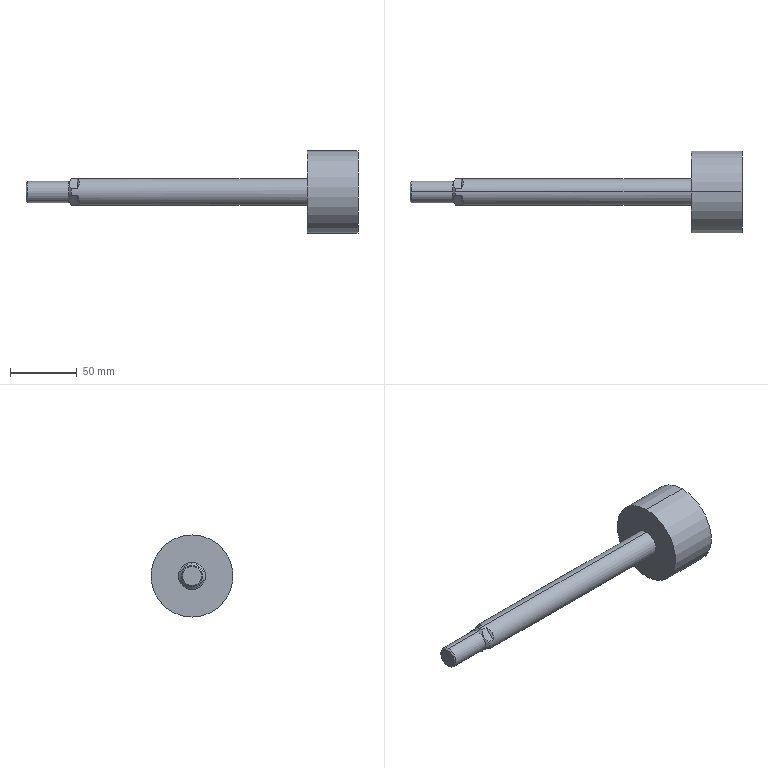Part | SolidWorks | features BaseBody 1 | 1 solid | 21 faces | box 248.5 x 61.5 x 61.5 mm | volume 175012 mm3 | plane 11 | cylinder 6 | cone 4 | commonest cylinder face diameters 16 x2 20 x2 61.5 x2
STEP:
#1=CARTESIAN_POINT('',(-37.,0.,-8.));
#2=VERTEX_POINT('',#1);
#3=CARTESIAN_POINT('',(-37.,0.,8.));
#4=VERTEX_POINT('',#3);
#5=CARTESIAN_POINT('',(-37.,0.,0.));
#6=DIRECTION('',(1.,0.,0.));
#7=DIRECTION('',(0.,0.,-1.));
#8=AXIS2_PLACEMENT_3D('',#5,#6,#7);
#9=CIRCLE('',#8,8.);
#10=EDGE_CURVE('',#2,#4,#9,.T.);
#11=ORIENTED_EDGE('',*,*,#10,.T.);
#12=CARTESIAN_POINT('',(-35.,0.,10.));
#13=VERTEX_POINT('',#12);
#14=CARTESIAN_POINT('',(-37.,0.,8.));
#15=DIRECTION('',(0.7071,0.,0.7071));
#16=VECTOR('',#15,1000.);
#17=LINE('',#14,#16);
#18=EDGE_CURVE('',#4,#13,#17,.T.);
#19=ORIENTED_EDGE('',*,*,#18,.T.);
#20=CARTESIAN_POINT('',(-35.,2.285,9.735));
#21=VERTEX_POINT('',#20);
#22=CARTESIAN_POINT('',(-35.,0.,0.));
#23=DIRECTION('',(1.,0.,0.));
#24=DIRECTION('',(0.,0.,-1.));
#25=AXIS2_PLACEMENT_3D('',#22,#23,#24);
#26=CIRCLE('',#25,10.);
#27=EDGE_CURVE('',#21,#13,#26,.T.);
#28=ORIENTED_EDGE('',*,*,#27,.F.);
#29=CARTESIAN_POINT('',(-35.,9.735,2.285));
#30=VERTEX_POINT('',#29);
#31=CARTESIAN_POINT('',(-35.,9.735,2.285));
#32=CARTESIAN_POINT('',(-35.236,9.419,2.602));
#33=CARTESIAN_POINT('',(-35.546,8.958,3.063));
#34=CARTESIAN_POINT('',(-35.834,8.441,3.58));
#35=CARTESIAN_POINT('',(-35.96,8.189,3.832));
#36=CARTESIAN_POINT('',(-36.018,8.064,3.957));
#37=CARTESIAN_POINT('',(-36.046,8.001,4.019));
#38=CARTESIAN_POINT('',(-36.057,7.975,4.046));
#39=CARTESIAN_POINT('',(-36.065,7.957,4.064));
#40=CARTESIAN_POINT('',(-36.068,7.95,4.071));
#41=CARTESIAN_POINT('',(-36.357,7.281,4.74));
#42=CARTESIAN_POINT('',(-36.5,6.638,5.383));
#43=CARTESIAN_POINT('',(-36.5,5.698,6.323));
#44=CARTESIAN_POINT('',(-36.447,5.221,6.799));
#45=CARTESIAN_POINT('',(-36.291,4.655,7.365));
#46=CARTESIAN_POINT('',(-36.19,4.37,7.651));
#47=CARTESIAN_POINT('',(-36.134,4.226,7.795));
#48=CARTESIAN_POINT('',(-36.104,4.154,7.866));
#49=CARTESIAN_POINT('',(-36.091,4.124,7.897));
#50=CARTESIAN_POINT('',(-36.082,4.103,7.918));
#51=CARTESIAN_POINT('',(-36.077,4.091,7.93));
#52=CARTESIAN_POINT('',(-35.829,3.517,8.503));
#53=CARTESIAN_POINT('',(-35.472,2.919,9.102));
#54=CARTESIAN_POINT('',(-35.,2.285,9.735));
#55=B_SPLINE_CURVE_WITH_KNOTS('',3,(#31,#32,#33,#34,#35,#36,#37,#38,#39,#40,#41,#42,#43,#44,#45,#46,#47,#48,#49,#50,#51,#52,#53,#54),.UNSPECIFIED.,.F.,.F.,(4,1,1,1,1,1,2,2,2,1,1,1,1,1,2,2,4),(0.,0.125,0.1875,0.2188,0.2344,0.2422,0.2461,0.25,0.5,0.625,0.6875,0.7188,0.7344,0.7422,0.7461,0.75,1.),.UNSPECIFIED.);
#56=EDGE_CURVE('',#30,#21,#55,.T.);
#57=ORIENTED_EDGE('',*,*,#56,.F.);
#58=CARTESIAN_POINT('',(-35.,9.735,-2.285));
#59=VERTEX_POINT('',#58);
#60=CARTESIAN_POINT('',(-35.,0.,0.));
#61=DIRECTION('',(1.,0.,0.));
#62=DIRECTION('',(0.,0.,-1.));
#63=AXIS2_PLACEMENT_3D('',#60,#61,#62);
#64=CIRCLE('',#63,10.);
#65=EDGE_CURVE('',#59,#30,#64,.T.);
#66=ORIENTED_EDGE('',*,*,#65,.F.);
#67=CARTESIAN_POINT('',(-35.,2.285,-9.735));
#68=VERTEX_POINT('',#67);
#69=CARTESIAN_POINT('',(-35.,2.285,-9.735));
#70=CARTESIAN_POINT('',(-35.236,2.602,-9.419));
#71=CARTESIAN_POINT('',(-35.546,3.063,-8.958));
#72=CARTESIAN_POINT('',(-35.834,3.58,-8.441));
#73=CARTESIAN_POINT('',(-35.96,3.832,-8.189));
#74=CARTESIAN_POINT('',(-36.018,3.957,-8.064));
#75=CARTESIAN_POINT('',(-36.046,4.019,-8.001));
#76=CARTESIAN_POINT('',(-36.057,4.046,-7.975));
#77=CARTESIAN_POINT('',(-36.065,4.064,-7.957));
#78=CARTESIAN_POINT('',(-36.068,4.071,-7.95));
#79=CARTESIAN_POINT('',(-36.357,4.74,-7.281));
#80=CARTESIAN_POINT('',(-36.5,5.383,-6.638));
#81=CARTESIAN_POINT('',(-36.5,6.323,-5.698));
#82=CARTESIAN_POINT('',(-36.447,6.799,-5.221));
#83=CARTESIAN_POINT('',(-36.291,7.365,-4.655));
#84=CARTESIAN_POINT('',(-36.19,7.651,-4.37));
#85=CARTESIAN_POINT('',(-36.134,7.795,-4.226));
#86=CARTESIAN_POINT('',(-36.104,7.866,-4.154));
#87=CARTESIAN_POINT('',(-36.091,7.897,-4.124));
#88=CARTESIAN_POINT('',(-36.082,7.918,-4.103));
#89=CARTESIAN_POINT('',(-36.077,7.93,-4.091));
#90=CARTESIAN_POINT('',(-35.829,8.503,-3.517));
#91=CARTESIAN_POINT('',(-35.472,9.102,-2.919));
#92=CARTESIAN_POINT('',(-35.,9.735,-2.285));
#93=B_SPLINE_CURVE_WITH_KNOTS('',3,(#69,#70,#71,#72,#73,#74,#75,#76,#77,#78,#79,#80,#81,#82,#83,#84,#85,#86,#87,#88,#89,#90,#91,#92),.UNSPECIFIED.,.F.,.F.,(4,1,1,1,1,1,2,2,2,1,1,1,1,1,2,2,4),(0.,0.125,0.1875,0.2188,0.2344,0.2422,0.2461,0.25,0.5,0.625,0.6875,0.7188,0.7344,0.7422,0.7461,0.75,1.),.UNSPECIFIED.);
#94=EDGE_CURVE('',#68,#59,#93,.T.);
#95=ORIENTED_EDGE('',*,*,#94,.F.);
#96=CARTESIAN_POINT('',(-35.,0.,-10.));
#97=VERTEX_POINT('',#96);
#98=CARTESIAN_POINT('',(-35.,0.,0.));
#99=DIRECTION('',(1.,0.,0.));
#100=DIRECTION('',(0.,0.,-1.));
#101=AXIS2_PLACEMENT_3D('',#98,#99,#100);
#102=CIRCLE('',#101,10.);
#103=EDGE_CURVE('',#97,#68,#102,.T.);
#104=ORIENTED_EDGE('',*,*,#103,.F.);
#105=CARTESIAN_POINT('',(-37.,0.,-8.));
#106=DIRECTION('',(0.7071,0.,-0.7071));
#107=VECTOR('',#106,1000.);
#108=LINE('',#105,#107);
#109=EDGE_CURVE('',#2,#97,#108,.T.);
#110=ORIENTED_EDGE('',*,*,#109,.F.);
#111=EDGE_LOOP('',(#11,#19,#28,#57,#66,#95,#104,#110));
#112=FACE_OUTER_BOUND('',#111,.T.);
#113=CARTESIAN_POINT('',(-37.,0.,0.));
#114=DIRECTION('',(1.,0.,0.));
#115=DIRECTION('',(0.,0.,-1.));
#116=AXIS2_PLACEMENT_3D('',#113,#114,#115);
#117=CONICAL_SURFACE('',#116,8.,0.7854);
#118=ADVANCED_FACE('',(#112),#117,.T.);
#119=CARTESIAN_POINT('',(141.5,0.,10.));
#120=VERTEX_POINT('',#119);
#121=CARTESIAN_POINT('',(141.5,0.,-10.));
#122=VERTEX_POINT('',#121);
#123=CARTESIAN_POINT('',(141.5,0.,0.));
#124=DIRECTION('',(1.,0.,0.));
#125=DIRECTION('',(0.,0.,-1.));
#126=AXIS2_PLACEMENT_3D('',#123,#124,#125);
#127=CIRCLE('',#126,10.);
#128=EDGE_CURVE('',#120,#122,#127,.T.);
#129=ORIENTED_EDGE('',*,*,#128,.F.);
#130=CARTESIAN_POINT('',(179.5,0.,10.));
#131=DIRECTION('',(-1.,0.,0.));
#132=VECTOR('',#131,1000.);
#133=LINE('',#130,#132);
#134=EDGE_CURVE('',#120,#13,#133,.T.);
#135=ORIENTED_EDGE('',*,*,#134,.T.);
#136=CARTESIAN_POINT('',(-35.,-2.285,9.735));
#137=VERTEX_POINT('',#136);
#138=CARTESIAN_POINT('',(-35.,0.,0.));
#139=DIRECTION('',(1.,0.,0.));
#140=DIRECTION('',(0.,0.,-1.));
#141=AXIS2_PLACEMENT_3D('',#138,#139,#140);
#142=CIRCLE('',#141,10.);
#143=EDGE_CURVE('',#13,#137,#142,.T.);
#144=ORIENTED_EDGE('',*,*,#143,.T.);
#145=CARTESIAN_POINT('',(-30.5,-2.285,9.735));
#146=VERTEX_POINT('',#145);
#147=CARTESIAN_POINT('',(179.5,-2.285,9.735));
#148=DIRECTION('',(-1.,0.,0.));
#149=VECTOR('',#148,1000.);
#150=LINE('',#147,#149);
#151=EDGE_CURVE('',#146,#137,#150,.T.);
#152=ORIENTED_EDGE('',*,*,#151,.F.);
#153=CARTESIAN_POINT('',(-30.5,-9.735,2.285));
#154=VERTEX_POINT('',#153);
#155=CARTESIAN_POINT('',(-30.5,-9.735,2.285));
#156=CARTESIAN_POINT('',(-28.444,-8.844,6.084));
#157=CARTESIAN_POINT('',(-28.444,-6.084,8.844));
#158=CARTESIAN_POINT('',(-30.5,-2.285,9.735));
#159=(BOUNDED_CURVE()B_SPLINE_CURVE(3,(#155,#156,#157,#158),.UNSPECIFIED.,.F.,.F.)B_SPLINE_CURVE_WITH_KNOTS((4,4),(5.728,6.838),.UNSPECIFIED.)CURVE()GEOMETRIC_REPRESENTATION_ITEM()RATIONAL_B_SPLINE_CURVE((1.,0.9,0.9,1.))REPRESENTATION_ITEM(''));
#160=EDGE_CURVE('',#154,#146,#159,.T.);
#161=ORIENTED_EDGE('',*,*,#160,.F.);
#162=CARTESIAN_POINT('',(-35.,-9.735,2.285));
#163=VERTEX_POINT('',#162);
#164=CARTESIAN_POINT('',(179.5,-9.735,2.285));
#165=DIRECTION('',(1.,0.,0.));
#166=VECTOR('',#165,1000.);
#167=LINE('',#164,#166);
#168=EDGE_CURVE('',#163,#154,#167,.T.);
#169=ORIENTED_EDGE('',*,*,#168,.F.);
#170=CARTESIAN_POINT('',(-35.,-9.735,-2.285));
#171=VERTEX_POINT('',#170);
#172=CARTESIAN_POINT('',(-35.,0.,0.));
#173=DIRECTION('',(1.,0.,0.));
#174=DIRECTION('',(0.,0.,-1.));
#175=AXIS2_PLACEMENT_3D('',#172,#173,#174);
#176=CIRCLE('',#175,10.);
#177=EDGE_CURVE('',#163,#171,#176,.T.);
#178=ORIENTED_EDGE('',*,*,#177,.T.);
#179=CARTESIAN_POINT('',(-30.5,-9.735,-2.285));
#180=VERTEX_POINT('',#179);
#181=CARTESIAN_POINT('',(179.5,-9.735,-2.285));
#182=DIRECTION('',(-1.,0.,0.));
#183=VECTOR('',#182,1000.);
#184=LINE('',#181,#183);
#185=EDGE_CURVE('',#180,#171,#184,.T.);
#186=ORIENTED_EDGE('',*,*,#185,.F.);
#187=CARTESIAN_POINT('',(-30.5,-2.285,-9.735));
#188=VERTEX_POINT('',#187);
#189=CARTESIAN_POINT('',(-30.5,-2.285,-9.735));
#190=CARTESIAN_POINT('',(-28.444,-6.084,-8.844));
#191=CARTESIAN_POINT('',(-28.444,-8.844,-6.084));
#192=CARTESIAN_POINT('',(-30.5,-9.735,-2.285));
#193=(BOUNDED_CURVE()B_SPLINE_CURVE(3,(#189,#190,#191,#192),.UNSPECIFIED.,.F.,.F.)B_SPLINE_CURVE_WITH_KNOTS((4,4),(5.728,6.838),.UNSPECIFIED.)CURVE()GEOMETRIC_REPRESENTATION_ITEM()RATIONAL_B_SPLINE_CURVE((1.,0.9,0.9,1.))REPRESENTATION_ITEM(''));
#194=EDGE_CURVE('',#188,#180,#193,.T.);
#195=ORIENTED_EDGE('',*,*,#194,.F.);
#196=CARTESIAN_POINT('',(-35.,-2.285,-9.735));
#197=VERTEX_POINT('',#196);
#198=CARTESIAN_POINT('',(179.5,-2.285,-9.735));
#199=DIRECTION('',(1.,0.,0.));
#200=VECTOR('',#199,1000.);
#201=LINE('',#198,#200);
#202=EDGE_CURVE('',#197,#188,#201,.T.);
#203=ORIENTED_EDGE('',*,*,#202,.F.);
#204=CARTESIAN_POINT('',(-35.,0.,0.));
#205=DIRECTION('',(1.,0.,0.));
#206=DIRECTION('',(0.,0.,-1.));
#207=AXIS2_PLACEMENT_3D('',#204,#205,#206);
#208=CIRCLE('',#207,10.);
#209=EDGE_CURVE('',#197,#97,#208,.T.);
#210=ORIENTED_EDGE('',*,*,#209,.T.);
#211=CARTESIAN_POINT('',(179.5,0.,-10.));
#212=DIRECTION('',(-1.,0.,0.));
#213=VECTOR('',#212,1000.);
#214=LINE('',#211,#213);
#215=EDGE_CURVE('',#122,#97,#214,.T.);
#216=ORIENTED_EDGE('',*,*,#215,.F.);
#217=EDGE_LOOP('',(#129,#135,#144,#152,#161,#169,#178,#186,#195,#203,#210,#216));
#218=FACE_OUTER_BOUND('',#217,.T.);
#219=CARTESIAN_POINT('',(179.5,0.,0.));
#220=DIRECTION('',(-1.,0.,0.));
#221=DIRECTION('',(0.,0.,-1.));
#222=AXIS2_PLACEMENT_3D('',#219,#220,#221);
#223=CYLINDRICAL_SURFACE('',#222,10.);
#224=ADVANCED_FACE('',(#218),#223,.T.);
#225=CARTESIAN_POINT('',(179.5,0.,30.75));
#226=VERTEX_POINT('',#225);
#227=CARTESIAN_POINT('',(179.5,0.,-30.75));
#228=VERTEX_POINT('',#227);
#229=CARTESIAN_POINT('',(179.5,0.,0.));
#230=DIRECTION('',(1.,0.,0.));
#231=DIRECTION('',(0.,0.,-1.));
#232=AXIS2_PLACEMENT_3D('',#229,#230,#231);
#233=CIRCLE('',#232,30.75);
#234=EDGE_CURVE('',#226,#228,#233,.T.);
#235=ORIENTED_EDGE('',*,*,#234,.F.);
#236=CARTESIAN_POINT('',(141.5,0.,30.75));
#237=VERTEX_POINT('',#236);
#238=CARTESIAN_POINT('',(179.5,0.,30.75));
#239=DIRECTION('',(-1.,0.,0.));
#240=VECTOR('',#239,1000.);
#241=LINE('',#238,#240);
#242=EDGE_CURVE('',#226,#237,#241,.T.);
#243=ORIENTED_EDGE('',*,*,#242,.T.);
#244=CARTESIAN_POINT('',(141.5,0.,-30.75));
#245=VERTEX_POINT('',#244);
#246=CARTESIAN_POINT('',(141.5,0.,0.));
#247=DIRECTION('',(1.,0.,0.));
#248=DIRECTION('',(0.,0.,-1.));
#249=AXIS2_PLACEMENT_3D('',#246,#247,#248);
#250=CIRCLE('',#249,30.75);
#251=EDGE_CURVE('',#237,#245,#250,.T.);
#252=ORIENTED_EDGE('',*,*,#251,.T.);
#253=CARTESIAN_POINT('',(179.5,0.,-30.75));
#254=DIRECTION('',(-1.,0.,0.));
#255=VECTOR('',#254,1000.);
#256=LINE('',#253,#255);
#257=EDGE_CURVE('',#228,#245,#256,.T.);
#258=ORIENTED_EDGE('',*,*,#257,.F.);
#259=EDGE_LOOP('',(#235,#243,#252,#258));
#260=FACE_OUTER_BOUND('',#259,.T.);
#261=CARTESIAN_POINT('',(179.5,0.,0.));
#262=DIRECTION('',(-1.,0.,0.));
#263=DIRECTION('',(0.,0.,-1.));
#264=AXIS2_PLACEMENT_3D('',#261,#262,#263);
#265=CYLINDRICAL_SURFACE('',#264,30.75);
#266=ADVANCED_FACE('',(#260),#265,.T.);
#267=CARTESIAN_POINT('',(-37.,0.,0.));
#268=DIRECTION('',(1.,0.,0.));
#269=DIRECTION('',(0.,0.,-1.));
#270=AXIS2_PLACEMENT_3D('',#267,#268,#269);
#271=CIRCLE('',#270,8.);
#272=EDGE_CURVE('',#4,#2,#271,.T.);
#273=ORIENTED_EDGE('',*,*,#272,.F.);
#274=CARTESIAN_POINT('',(-68.08,0.,8.));
#275=VERTEX_POINT('',#274);
#276=CARTESIAN_POINT('',(179.5,0.,8.));
#277=DIRECTION('',(-1.,0.,0.));
#278=VECTOR('',#277,1000.);
#279=LINE('',#276,#278);
#280=EDGE_CURVE('',#4,#275,#279,.T.);
#281=ORIENTED_EDGE('',*,*,#280,.T.);
#282=CARTESIAN_POINT('',(-68.08,0.,-8.));
#283=VERTEX_POINT('',#282);
#284=CARTESIAN_POINT('',(-68.08,0.,0.));
#285=DIRECTION('',(1.,0.,0.));
#286=DIRECTION('',(0.,0.,-1.));
#287=AXIS2_PLACEMENT_3D('',#284,#285,#286);
#288=CIRCLE('',#287,8.);
#289=EDGE_CURVE('',#275,#283,#288,.T.);
#290=ORIENTED_EDGE('',*,*,#289,.T.);
#291=CARTESIAN_POINT('',(179.5,0.,-8.));
#292=DIRECTION('',(-1.,0.,0.));
#293=VECTOR('',#292,1000.);
#294=LINE('',#291,#293);
#295=EDGE_CURVE('',#2,#283,#294,.T.);
#296=ORIENTED_EDGE('',*,*,#295,.F.);
#297=EDGE_LOOP('',(#273,#281,#290,#296));
#298=FACE_OUTER_BOUND('',#297,.T.);
#299=CARTESIAN_POINT('',(179.5,0.,0.));
#300=DIRECTION('',(-1.,0.,0.));
#301=DIRECTION('',(0.,0.,-1.));
#302=AXIS2_PLACEMENT_3D('',#299,#300,#301);
#303=CYLINDRICAL_SURFACE('',#302,8.);
#304=ADVANCED_FACE('',(#298),#303,.T.);
#305=CARTESIAN_POINT('',(-69.,0.,-7.08));
#306=VERTEX_POINT('',#305);
#307=CARTESIAN_POINT('',(-69.,0.,7.08));
#308=VERTEX_POINT('',#307);
#309=CARTESIAN_POINT('',(-69.,0.,0.));
#310=DIRECTION('',(1.,0.,0.));
#311=DIRECTION('',(0.,0.,-1.));
#312=AXIS2_PLACEMENT_3D('',#309,#310,#311);
#313=CIRCLE('',#312,7.08);
#314=EDGE_CURVE('',#306,#308,#313,.T.);
#315=ORIENTED_EDGE('',*,*,#314,.T.);
#316=CARTESIAN_POINT('',(-69.,0.,7.08));
#317=DIRECTION('',(0.7071,0.,0.7071));
#318=VECTOR('',#317,1000.);
#319=LINE('',#316,#318);
#320=EDGE_CURVE('',#308,#275,#319,.T.);
#321=ORIENTED_EDGE('',*,*,#320,.T.);
#322=CARTESIAN_POINT('',(-68.08,0.,0.));
#323=DIRECTION('',(1.,0.,0.));
#324=DIRECTION('',(0.,0.,-1.));
#325=AXIS2_PLACEMENT_3D('',#322,#323,#324);
#326=CIRCLE('',#325,8.);
#327=EDGE_CURVE('',#283,#275,#326,.T.);
#328=ORIENTED_EDGE('',*,*,#327,.F.);
#329=CARTESIAN_POINT('',(-69.,0.,-7.08));
#330=DIRECTION('',(0.7071,0.,-0.7071));
#331=VECTOR('',#330,1000.);
#332=LINE('',#329,#331);
#333=EDGE_CURVE('',#306,#283,#332,.T.);
#334=ORIENTED_EDGE('',*,*,#333,.F.);
#335=EDGE_LOOP('',(#315,#321,#328,#334));
#336=FACE_OUTER_BOUND('',#335,.T.);
#337=CARTESIAN_POINT('',(-69.,0.,0.));
#338=DIRECTION('',(1.,0.,0.));
#339=DIRECTION('',(0.,0.,-1.));
#340=AXIS2_PLACEMENT_3D('',#337,#338,#339);
#341=CONICAL_SURFACE('',#340,7.08,0.7854);
#342=ADVANCED_FACE('',(#336),#341,.T.);
#343=CARTESIAN_POINT('',(-30.5,2.285,9.735));
#344=VERTEX_POINT('',#343);
#345=CARTESIAN_POINT('',(179.5,2.285,9.735));
#346=DIRECTION('',(1.,0.,0.));
#347=VECTOR('',#346,1000.);
#348=LINE('',#345,#347);
#349=EDGE_CURVE('',#21,#344,#348,.T.);
#350=ORIENTED_EDGE('',*,*,#349,.T.);
#351=CARTESIAN_POINT('',(-30.5,9.735,2.285));
#352=VERTEX_POINT('',#351);
#353=CARTESIAN_POINT('',(-30.5,0.,12.021));
#354=DIRECTION('',(0.,0.7071,-0.7071));
#355=VECTOR('',#354,1000.);
#356=LINE('',#353,#355);
#357=EDGE_CURVE('',#344,#352,#356,.T.);
#358=ORIENTED_EDGE('',*,*,#357,.T.);
#359=CARTESIAN_POINT('',(179.5,9.735,2.285));
#360=DIRECTION('',(-1.,0.,0.));
#361=VECTOR('',#360,1000.);
#362=LINE('',#359,#361);
#363=EDGE_CURVE('',#352,#30,#362,.T.);
#364=ORIENTED_EDGE('',*,*,#363,.T.);
#365=ORIENTED_EDGE('',*,*,#56,.T.);
#366=EDGE_LOOP('',(#350,#358,#364,#365));
#367=FACE_OUTER_BOUND('',#366,.T.);
#368=CARTESIAN_POINT('',(-71.7,0.,12.021));
#369=DIRECTION('',(0.,0.7071,0.7071));
#370=DIRECTION('',(1.,0.,0.));
#371=AXIS2_PLACEMENT_3D('',#368,#369,#370);
#372=PLANE('',#371);
#373=ADVANCED_FACE('',(#367),#372,.T.);
#374=CARTESIAN_POINT('',(-30.5,2.285,9.735));
#375=CARTESIAN_POINT('',(-28.444,6.084,8.844));
#376=CARTESIAN_POINT('',(-28.444,8.844,6.084));
#377=CARTESIAN_POINT('',(-30.5,9.735,2.285));
#378=(BOUNDED_CURVE()B_SPLINE_CURVE(3,(#374,#375,#376,#377),.UNSPECIFIED.,.F.,.F.)B_SPLINE_CURVE_WITH_KNOTS((4,4),(5.728,6.838),.UNSPECIFIED.)CURVE()GEOMETRIC_REPRESENTATION_ITEM()RATIONAL_B_SPLINE_CURVE((1.,0.9,0.9,1.))REPRESENTATION_ITEM(''));
#379=EDGE_CURVE('',#344,#352,#378,.T.);
#380=ORIENTED_EDGE('',*,*,#379,.T.);
#381=ORIENTED_EDGE('',*,*,#357,.F.);
#382=EDGE_LOOP('',(#380,#381));
#383=FACE_OUTER_BOUND('',#382,.T.);
#384=CARTESIAN_POINT('',(-30.5,0.,12.021));
#385=DIRECTION('',(-0.7071,0.5,0.5));
#386=DIRECTION('',(0.5774,0.,0.8165));
#387=AXIS2_PLACEMENT_3D('',#384,#385,#386);
#388=PLANE('',#387);
#389=ADVANCED_FACE('',(#383),#388,.T.);
#390=ORIENTED_EDGE('',*,*,#320,.F.);
#391=CARTESIAN_POINT('',(-69.,0.,0.));
#392=DIRECTION('',(1.,0.,0.));
#393=DIRECTION('',(0.,0.,-1.));
#394=AXIS2_PLACEMENT_3D('',#391,#392,#393);
#395=CIRCLE('',#394,7.08);
#396=EDGE_CURVE('',#308,#306,#395,.T.);
#397=ORIENTED_EDGE('',*,*,#396,.T.);
#398=ORIENTED_EDGE('',*,*,#333,.T.);
#399=ORIENTED_EDGE('',*,*,#289,.F.);
#400=EDGE_LOOP('',(#390,#397,#398,#399));
#401=FACE_OUTER_BOUND('',#400,.T.);
#402=CARTESIAN_POINT('',(-69.,0.,0.));
#403=DIRECTION('',(1.,0.,0.));
#404=DIRECTION('',(0.,0.,-1.));
#405=AXIS2_PLACEMENT_3D('',#402,#403,#404);
#406=CONICAL_SURFACE('',#405,7.08,0.7854);
#407=ADVANCED_FACE('',(#401),#406,.T.);
#408=ORIENTED_EDGE('',*,*,#280,.F.);
#409=ORIENTED_EDGE('',*,*,#10,.F.);
#410=ORIENTED_EDGE('',*,*,#295,.T.);
#411=ORIENTED_EDGE('',*,*,#327,.T.);
#412=EDGE_LOOP('',(#408,#409,#410,#411));
#413=FACE_OUTER_BOUND('',#412,.T.);
#414=CARTESIAN_POINT('',(179.5,0.,0.));
#415=DIRECTION('',(-1.,0.,0.));
#416=DIRECTION('',(0.,0.,-1.));
#417=AXIS2_PLACEMENT_3D('',#414,#415,#416);
#418=CYLINDRICAL_SURFACE('',#417,8.);
#419=ADVANCED_FACE('',(#413),#418,.T.);
#420=CARTESIAN_POINT('',(179.5,0.,0.));
#421=DIRECTION('',(1.,0.,0.));
#422=DIRECTION('',(0.,0.,-1.));
#423=AXIS2_PLACEMENT_3D('',#420,#421,#422);
#424=CIRCLE('',#423,30.75);
#425=EDGE_CURVE('',#228,#226,#424,.T.);
#426=ORIENTED_EDGE('',*,*,#425,.T.);
#427=ORIENTED_EDGE('',*,*,#234,.T.);
#428=EDGE_LOOP('',(#426,#427));
#429=FACE_OUTER_BOUND('',#428,.T.);
#430=CARTESIAN_POINT('',(179.5,30.75,0.));
#431=DIRECTION('',(-1.,0.,0.));
#432=DIRECTION('',(0.,0.,1.));
#433=AXIS2_PLACEMENT_3D('',#430,#431,#432);
#434=PLANE('',#433);
#435=ADVANCED_FACE('',(#429),#434,.F.);
#436=ORIENTED_EDGE('',*,*,#242,.F.);
#437=ORIENTED_EDGE('',*,*,#425,.F.);
#438=ORIENTED_EDGE('',*,*,#257,.T.);
#439=CARTESIAN_POINT('',(141.5,0.,0.));
#440=DIRECTION('',(1.,0.,0.));
#441=DIRECTION('',(0.,0.,-1.));
#442=AXIS2_PLACEMENT_3D('',#439,#440,#441);
#443=CIRCLE('',#442,30.75);
#444=EDGE_CURVE('',#245,#237,#443,.T.);
#445=ORIENTED_EDGE('',*,*,#444,.T.);
#446=EDGE_LOOP('',(#436,#437,#438,#445));
#447=FACE_OUTER_BOUND('',#446,.T.);
#448=CARTESIAN_POINT('',(179.5,0.,0.));
#449=DIRECTION('',(-1.,0.,0.));
#450=DIRECTION('',(0.,0.,-1.));
#451=AXIS2_PLACEMENT_3D('',#448,#449,#450);
#452=CYLINDRICAL_SURFACE('',#451,30.75);
#453=ADVANCED_FACE('',(#447),#452,.T.);
#454=CARTESIAN_POINT('',(141.5,0.,0.));
#455=DIRECTION('',(1.,0.,0.));
#456=DIRECTION('',(0.,0.,-1.));
#457=AXIS2_PLACEMENT_3D('',#454,#455,#456);
#458=CIRCLE('',#457,10.);
#459=EDGE_CURVE('',#122,#120,#458,.T.);
#460=ORIENTED_EDGE('',*,*,#459,.T.);
#461=ORIENTED_EDGE('',*,*,#128,.T.);
#462=EDGE_LOOP('',(#460,#461));
#463=FACE_BOUND('',#462,.T.);
#464=ORIENTED_EDGE('',*,*,#444,.F.);
#465=ORIENTED_EDGE('',*,*,#251,.F.);
#466=EDGE_LOOP('',(#464,#465));
#467=FACE_OUTER_BOUND('',#466,.T.);
#468=CARTESIAN_POINT('',(141.5,10.,0.));
#469=DIRECTION('',(1.,0.,0.));
#470=DIRECTION('',(0.,1.,0.));
#471=AXIS2_PLACEMENT_3D('',#468,#469,#470);
#472=PLANE('',#471);
#473=ADVANCED_FACE('',(#463,#467),#472,.F.);
#474=ORIENTED_EDGE('',*,*,#314,.F.);
#475=ORIENTED_EDGE('',*,*,#396,.F.);
#476=EDGE_LOOP('',(#474,#475));
#477=FACE_OUTER_BOUND('',#476,.T.);
#478=CARTESIAN_POINT('',(-69.,0.,0.));
#479=DIRECTION('',(1.,0.,0.));
#480=DIRECTION('',(0.,1.,0.));
#481=AXIS2_PLACEMENT_3D('',#478,#479,#480);
#482=PLANE('',#481);
#483=ADVANCED_FACE('',(#477),#482,.F.);
#484=ORIENTED_EDGE('',*,*,#134,.F.);
#485=ORIENTED_EDGE('',*,*,#459,.F.);
#486=ORIENTED_EDGE('',*,*,#215,.T.);
#487=ORIENTED_EDGE('',*,*,#103,.T.);
#488=CARTESIAN_POINT('',(-30.5,2.285,-9.735));
#489=VERTEX_POINT('',#488);
#490=CARTESIAN_POINT('',(179.5,2.285,-9.735));
#491=DIRECTION('',(-1.,0.,0.));
#492=VECTOR('',#491,1000.);
#493=LINE('',#490,#492);
#494=EDGE_CURVE('',#489,#68,#493,.T.);
#495=ORIENTED_EDGE('',*,*,#494,.F.);
#496=CARTESIAN_POINT('',(-30.5,9.735,-2.285));
#497=VERTEX_POINT('',#496);
#498=CARTESIAN_POINT('',(-30.5,9.735,-2.285));
#499=CARTESIAN_POINT('',(-28.444,8.844,-6.084));
#500=CARTESIAN_POINT('',(-28.444,6.084,-8.844));
#501=CARTESIAN_POINT('',(-30.5,2.285,-9.735));
#502=(BOUNDED_CURVE()B_SPLINE_CURVE(3,(#498,#499,#500,#501),.UNSPECIFIED.,.F.,.F.)B_SPLINE_CURVE_WITH_KNOTS((4,4),(5.728,6.838),.UNSPECIFIED.)CURVE()GEOMETRIC_REPRESENTATION_ITEM()RATIONAL_B_SPLINE_CURVE((1.,0.9,0.9,1.))REPRESENTATION_ITEM(''));
#503=EDGE_CURVE('',#497,#489,#502,.T.);
#504=ORIENTED_EDGE('',*,*,#503,.F.);
#505=CARTESIAN_POINT('',(179.5,9.735,-2.285));
#506=DIRECTION('',(1.,0.,0.));
#507=VECTOR('',#506,1000.);
#508=LINE('',#505,#507);
#509=EDGE_CURVE('',#59,#497,#508,.T.);
#510=ORIENTED_EDGE('',*,*,#509,.F.);
#511=ORIENTED_EDGE('',*,*,#65,.T.);
#512=ORIENTED_EDGE('',*,*,#363,.F.);
#513=ORIENTED_EDGE('',*,*,#379,.F.);
#514=ORIENTED_EDGE('',*,*,#349,.F.);
#515=ORIENTED_EDGE('',*,*,#27,.T.);
#516=EDGE_LOOP('',(#484,#485,#486,#487,#495,#504,#510,#511,#512,#513,#514,#515));
#517=FACE_OUTER_BOUND('',#516,.T.);
#518=CARTESIAN_POINT('',(179.5,0.,0.));
#519=DIRECTION('',(-1.,0.,0.));
#520=DIRECTION('',(0.,0.,-1.));
#521=AXIS2_PLACEMENT_3D('',#518,#519,#520);
#522=CYLINDRICAL_SURFACE('',#521,10.);
#523=ADVANCED_FACE('',(#517),#522,.T.);
#524=ORIENTED_EDGE('',*,*,#18,.F.);
#525=ORIENTED_EDGE('',*,*,#272,.T.);
#526=ORIENTED_EDGE('',*,*,#109,.T.);
#527=ORIENTED_EDGE('',*,*,#209,.F.);
#528=CARTESIAN_POINT('',(-35.,-9.735,-2.285));
#529=CARTESIAN_POINT('',(-35.236,-9.419,-2.602));
#530=CARTESIAN_POINT('',(-35.546,-8.958,-3.063));
#531=CARTESIAN_POINT('',(-35.834,-8.441,-3.58));
#532=CARTESIAN_POINT('',(-35.96,-8.189,-3.832));
#533=CARTESIAN_POINT('',(-36.018,-8.064,-3.957));
#534=CARTESIAN_POINT('',(-36.046,-8.001,-4.019));
#535=CARTESIAN_POINT('',(-36.057,-7.975,-4.046));
#536=CARTESIAN_POINT('',(-36.065,-7.957,-4.064));
#537=CARTESIAN_POINT('',(-36.068,-7.95,-4.071));
#538=CARTESIAN_POINT('',(-36.357,-7.281,-4.74));
#539=CARTESIAN_POINT('',(-36.5,-6.638,-5.383));
#540=CARTESIAN_POINT('',(-36.5,-5.698,-6.323));
#541=CARTESIAN_POINT('',(-36.447,-5.221,-6.799));
#542=CARTESIAN_POINT('',(-36.291,-4.655,-7.365));
#543=CARTESIAN_POINT('',(-36.19,-4.37,-7.651));
#544=CARTESIAN_POINT('',(-36.134,-4.226,-7.795));
#545=CARTESIAN_POINT('',(-36.104,-4.154,-7.866));
#546=CARTESIAN_POINT('',(-36.091,-4.124,-7.897));
#547=CARTESIAN_POINT('',(-36.082,-4.103,-7.918));
#548=CARTESIAN_POINT('',(-36.077,-4.091,-7.93));
#549=CARTESIAN_POINT('',(-35.829,-3.517,-8.503));
#550=CARTESIAN_POINT('',(-35.472,-2.919,-9.102));
#551=CARTESIAN_POINT('',(-35.,-2.285,-9.735));
#552=B_SPLINE_CURVE_WITH_KNOTS('',3,(#528,#529,#530,#531,#532,#533,#534,#535,#536,#537,#538,#539,#540,#541,#542,#543,#544,#545,#546,#547,#548,#549,#550,#551),.UNSPECIFIED.,.F.,.F.,(4,1,1,1,1,1,2,2,2,1,1,1,1,1,2,2,4),(0.,0.125,0.1875,0.2188,0.2344,0.2422,0.2461,0.25,0.5,0.625,0.6875,0.7188,0.7344,0.7422,0.7461,0.75,1.),.UNSPECIFIED.);
#553=EDGE_CURVE('',#171,#197,#552,.T.);
#554=ORIENTED_EDGE('',*,*,#553,.F.);
#555=ORIENTED_EDGE('',*,*,#177,.F.);
#556=CARTESIAN_POINT('',(-35.,-2.285,9.735));
#557=CARTESIAN_POINT('',(-35.236,-2.602,9.419));
#558=CARTESIAN_POINT('',(-35.546,-3.063,8.958));
#559=CARTESIAN_POINT('',(-35.834,-3.58,8.441));
#560=CARTESIAN_POINT('',(-35.96,-3.832,8.189));
#561=CARTESIAN_POINT('',(-36.018,-3.957,8.064));
#562=CARTESIAN_POINT('',(-36.046,-4.019,8.001));
#563=CARTESIAN_POINT('',(-36.057,-4.046,7.975));
#564=CARTESIAN_POINT('',(-36.065,-4.064,7.957));
#565=CARTESIAN_POINT('',(-36.068,-4.071,7.95));
#566=CARTESIAN_POINT('',(-36.357,-4.74,7.281));
#567=CARTESIAN_POINT('',(-36.5,-5.383,6.638));
#568=CARTESIAN_POINT('',(-36.5,-6.323,5.698));
#569=CARTESIAN_POINT('',(-36.447,-6.799,5.221));
#570=CARTESIAN_POINT('',(-36.291,-7.365,4.655));
#571=CARTESIAN_POINT('',(-36.19,-7.651,4.37));
#572=CARTESIAN_POINT('',(-36.134,-7.795,4.226));
#573=CARTESIAN_POINT('',(-36.104,-7.866,4.154));
#574=CARTESIAN_POINT('',(-36.091,-7.897,4.124));
#575=CARTESIAN_POINT('',(-36.082,-7.918,4.103));
#576=CARTESIAN_POINT('',(-36.077,-7.93,4.091));
#577=CARTESIAN_POINT('',(-35.829,-8.503,3.517));
#578=CARTESIAN_POINT('',(-35.472,-9.102,2.919));
#579=CARTESIAN_POINT('',(-35.,-9.735,2.285));
#580=B_SPLINE_CURVE_WITH_KNOTS('',3,(#556,#557,#558,#559,#560,#561,#562,#563,#564,#565,#566,#567,#568,#569,#570,#571,#572,#573,#574,#575,#576,#577,#578,#579),.UNSPECIFIED.,.F.,.F.,(4,1,1,1,1,1,2,2,2,1,1,1,1,1,2,2,4),(0.,0.125,0.1875,0.2187,0.2344,0.2422,0.2461,0.25,0.5,0.625,0.6875,0.7187,0.7344,0.7422,0.7461,0.75,1.),.UNSPECIFIED.);
#581=EDGE_CURVE('',#137,#163,#580,.T.);
#582=ORIENTED_EDGE('',*,*,#581,.F.);
#583=ORIENTED_EDGE('',*,*,#143,.F.);
#584=EDGE_LOOP('',(#524,#525,#526,#527,#554,#555,#582,#583));
#585=FACE_OUTER_BOUND('',#584,.T.);
#586=CARTESIAN_POINT('',(-37.,0.,0.));
#587=DIRECTION('',(1.,0.,0.));
#588=DIRECTION('',(0.,0.,-1.));
#589=AXIS2_PLACEMENT_3D('',#586,#587,#588);
#590=CONICAL_SURFACE('',#589,8.,0.7854);
#591=ADVANCED_FACE('',(#585),#590,.T.);
#592=ORIENTED_EDGE('',*,*,#168,.T.);
#593=CARTESIAN_POINT('',(-30.5,0.,12.021));
#594=DIRECTION('',(0.,-0.7071,-0.7071));
#595=VECTOR('',#594,1000.);
#596=LINE('',#593,#595);
#597=EDGE_CURVE('',#146,#154,#596,.T.);
#598=ORIENTED_EDGE('',*,*,#597,.F.);
#599=ORIENTED_EDGE('',*,*,#151,.T.);
#600=ORIENTED_EDGE('',*,*,#581,.T.);
#601=EDGE_LOOP('',(#592,#598,#599,#600));
#602=FACE_OUTER_BOUND('',#601,.T.);
#603=CARTESIAN_POINT('',(-30.5,0.,12.021));
#604=DIRECTION('',(0.,-0.7071,0.7071));
#605=DIRECTION('',(-1.,0.,0.));
#606=AXIS2_PLACEMENT_3D('',#603,#604,#605);
#607=PLANE('',#606);
#608=ADVANCED_FACE('',(#602),#607,.T.);
#609=ORIENTED_EDGE('',*,*,#160,.T.);
#610=ORIENTED_EDGE('',*,*,#597,.T.);
#611=EDGE_LOOP('',(#609,#610));
#612=FACE_OUTER_BOUND('',#611,.T.);
#613=CARTESIAN_POINT('',(-29.,-1.061,13.081));
#614=DIRECTION('',(-0.7071,-0.5,0.5));
#615=DIRECTION('',(-0.5774,0.8165,0.));
#616=AXIS2_PLACEMENT_3D('',#613,#614,#615);
#617=PLANE('',#616);
#618=ADVANCED_FACE('',(#612),#617,.T.);
#619=ORIENTED_EDGE('',*,*,#509,.T.);
#620=CARTESIAN_POINT('',(-30.5,12.021,0.));
#621=DIRECTION('',(0.,-0.7071,-0.7071));
#622=VECTOR('',#621,1000.);
#623=LINE('',#620,#622);
#624=EDGE_CURVE('',#497,#489,#623,.T.);
#625=ORIENTED_EDGE('',*,*,#624,.T.);
#626=ORIENTED_EDGE('',*,*,#494,.T.);
#627=ORIENTED_EDGE('',*,*,#94,.T.);
#628=EDGE_LOOP('',(#619,#625,#626,#627));
#629=FACE_OUTER_BOUND('',#628,.T.);
#630=CARTESIAN_POINT('',(-71.7,12.021,0.));
#631=DIRECTION('',(0.,0.7071,-0.7071));
#632=DIRECTION('',(-1.,0.,0.));
#633=AXIS2_PLACEMENT_3D('',#630,#631,#632);
#634=PLANE('',#633);
#635=ADVANCED_FACE('',(#629),#634,.T.);
#636=ORIENTED_EDGE('',*,*,#503,.T.);
#637=ORIENTED_EDGE('',*,*,#624,.F.);
#638=EDGE_LOOP('',(#636,#637));
#639=FACE_OUTER_BOUND('',#638,.T.);
#640=CARTESIAN_POINT('',(-30.5,12.021,0.));
#641=DIRECTION('',(-0.7071,0.5,-0.5));
#642=DIRECTION('',(-0.5774,0.,0.8165));
#643=AXIS2_PLACEMENT_3D('',#640,#641,#642);
#644=PLANE('',#643);
#645=ADVANCED_FACE('',(#639),#644,.T.);
#646=ORIENTED_EDGE('',*,*,#194,.T.);
#647=CARTESIAN_POINT('',(-30.5,-12.021,0.));
#648=DIRECTION('',(0.,0.7071,-0.7071));
#649=VECTOR('',#648,1000.);
#650=LINE('',#647,#649);
#651=EDGE_CURVE('',#180,#188,#650,.T.);
#652=ORIENTED_EDGE('',*,*,#651,.T.);
#653=EDGE_LOOP('',(#646,#652));
#654=FACE_OUTER_BOUND('',#653,.T.);
#655=CARTESIAN_POINT('',(-29.,-13.081,-1.061));
#656=DIRECTION('',(-0.7071,-0.5,-0.5));
#657=DIRECTION('',(-0.5774,0.,0.8165));
#658=AXIS2_PLACEMENT_3D('',#655,#656,#657);
#659=PLANE('',#658);
#660=ADVANCED_FACE('',(#654),#659,.T.);
#661=ORIENTED_EDGE('',*,*,#202,.T.);
#662=ORIENTED_EDGE('',*,*,#651,.F.);
#663=ORIENTED_EDGE('',*,*,#185,.T.);
#664=ORIENTED_EDGE('',*,*,#553,.T.);
#665=EDGE_LOOP('',(#661,#662,#663,#664));
#666=FACE_OUTER_BOUND('',#665,.T.);
#667=CARTESIAN_POINT('',(-30.5,-12.021,0.));
#668=DIRECTION('',(0.,-0.7071,-0.7071));
#669=DIRECTION('',(0.,-0.7071,0.7071));
#670=AXIS2_PLACEMENT_3D('',#667,#668,#669);
#671=PLANE('',#670);
#672=ADVANCED_FACE('',(#666),#671,.T.);
#673=CLOSED_SHELL('',(#118,#224,#266,#304,#342,#373,#389,#407,#419,#435,#453,#473,#483,#523,#591,#608,#618,#635,#645,#660,#672));
#674=MANIFOLD_SOLID_BREP('',#673);
#675=CARTESIAN_POINT('',(0.,0.,0.));
#676=DIRECTION('',(0.,0.,1.));
#677=DIRECTION('',(1.,0.,0.));
#678=AXIS2_PLACEMENT_3D('',#675,#676,#677);
#679=(LENGTH_UNIT()NAMED_UNIT(*)SI_UNIT(.MILLI.,.METRE.));
#680=UNCERTAINTY_MEASURE_WITH_UNIT(LENGTH_MEASURE(0.00001),#679,'','');
#681=(NAMED_UNIT(*)PLANE_ANGLE_UNIT()SI_UNIT($,.RADIAN.));
#682=(NAMED_UNIT(*)SI_UNIT($,.STERADIAN.)SOLID_ANGLE_UNIT());
#683=(GEOMETRIC_REPRESENTATION_CONTEXT(3)GLOBAL_UNCERTAINTY_ASSIGNED_CONTEXT((#680))GLOBAL_UNIT_ASSIGNED_CONTEXT((#679,#681,#682))REPRESENTATION_CONTEXT('',''));
#684=ADVANCED_BREP_SHAPE_REPRESENTATION('',(#674,#678),#683);